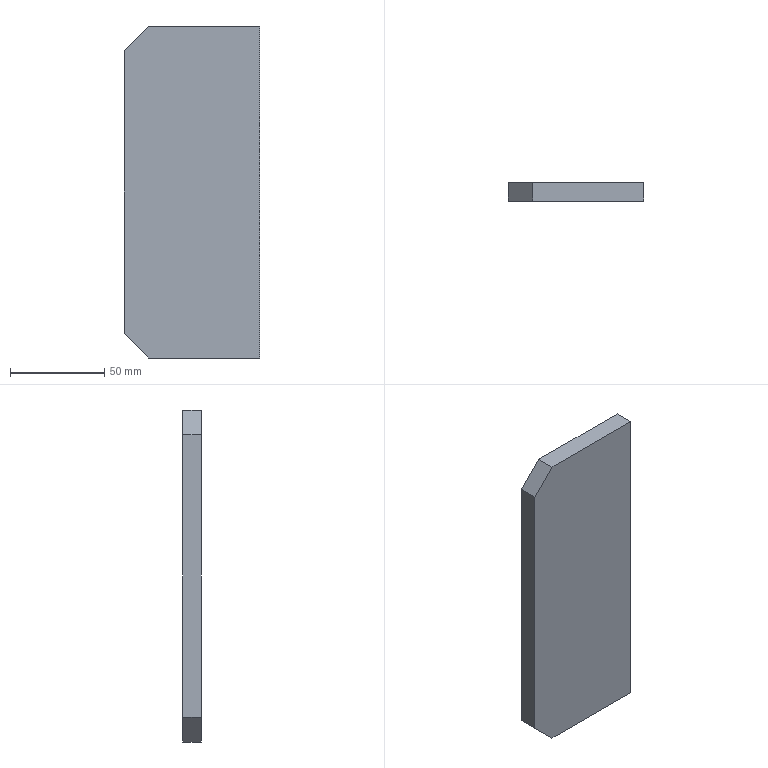Part | STEP file | 立柱填充筋Plate-194×150 | 1 solid | 8 faces | box 72 x 10 x 176 mm | volume 125030 mm3 | plane 8
STEP:
#1=CARTESIAN_POINT('',(0.,0.,0.));
#2=DIRECTION('',(0.,0.,1.));
#3=DIRECTION('',(1.,0.,0.));
#4=AXIS2_PLACEMENT_3D('',#1,#2,#3);
#5=CARTESIAN_POINT('',(72.,0.,88.));
#6=VERTEX_POINT('',#5);
#7=CARTESIAN_POINT('',(72.,0.,-88.));
#8=VERTEX_POINT('',#7);
#9=CARTESIAN_POINT('',(72.,0.,-88.));
#10=DIRECTION('',(0.,0.,-1.));
#11=VECTOR('',#10,1.);
#12=LINE('',#9,#11);
#13=CARTESIAN_POINT('',(72.,10.,-88.));
#14=DIRECTION('',(-1.,0.,0.));
#15=DIRECTION('',(0.,0.,1.));
#16=AXIS2_PLACEMENT_3D('',#13,#14,#15);
#17=PLANE('',#16);
#18=CARTESIAN_POINT('',(0.,-10.));
#19=DIRECTION('',(-1.,0.));
#20=VECTOR('',#19,1.);
#21=LINE('',#18,#20);
#22=(GEOMETRIC_REPRESENTATION_CONTEXT(2)PARAMETRIC_REPRESENTATION_CONTEXT()REPRESENTATION_CONTEXT('',''));
#23=DEFINITIONAL_REPRESENTATION('',(#21),#22);
#24=PCURVE('',#17,#23);
#25=CARTESIAN_POINT('',(0.,0.,0.));
#26=DIRECTION('',(0.,-1.,0.));
#27=DIRECTION('',(0.,0.,-1.));
#28=AXIS2_PLACEMENT_3D('',#25,#26,#27);
#29=PLANE('',#28);
#30=CARTESIAN_POINT('',(88.,72.));
#31=DIRECTION('',(1.,0.));
#32=VECTOR('',#31,1.);
#33=LINE('',#30,#32);
#34=(GEOMETRIC_REPRESENTATION_CONTEXT(2)PARAMETRIC_REPRESENTATION_CONTEXT()REPRESENTATION_CONTEXT('',''));
#35=DEFINITIONAL_REPRESENTATION('',(#33),#34);
#36=PCURVE('',#29,#35);
#37=SURFACE_CURVE('',#12,(#24,#36),.PCURVE_S1.);
#38=EDGE_CURVE('',#6,#8,#37,.T.);
#39=ORIENTED_EDGE('',*,*,#38,.T.);
#40=CARTESIAN_POINT('',(72.,10.,-88.));
#41=VERTEX_POINT('',#40);
#42=CARTESIAN_POINT('',(72.,10.,-88.));
#43=DIRECTION('',(0.,-1.,0.));
#44=VECTOR('',#43,1.);
#45=LINE('',#42,#44);
#46=CARTESIAN_POINT('',(0.,0.));
#47=DIRECTION('',(0.,-1.));
#48=VECTOR('',#47,1.);
#49=LINE('',#46,#48);
#50=(GEOMETRIC_REPRESENTATION_CONTEXT(2)PARAMETRIC_REPRESENTATION_CONTEXT()REPRESENTATION_CONTEXT('',''));
#51=DEFINITIONAL_REPRESENTATION('',(#49),#50);
#52=PCURVE('',#17,#51);
#53=CARTESIAN_POINT('',(0.,10.,-88.));
#54=DIRECTION('',(0.,0.,1.));
#55=DIRECTION('',(1.,0.,0.));
#56=AXIS2_PLACEMENT_3D('',#53,#54,#55);
#57=PLANE('',#56);
#58=CARTESIAN_POINT('',(72.,0.));
#59=DIRECTION('',(0.,-1.));
#60=VECTOR('',#59,1.);
#61=LINE('',#58,#60);
#62=(GEOMETRIC_REPRESENTATION_CONTEXT(2)PARAMETRIC_REPRESENTATION_CONTEXT()REPRESENTATION_CONTEXT('',''));
#63=DEFINITIONAL_REPRESENTATION('',(#61),#62);
#64=PCURVE('',#57,#63);
#65=SURFACE_CURVE('',#45,(#52,#64),.PCURVE_S1.);
#66=EDGE_CURVE('',#41,#8,#65,.T.);
#67=ORIENTED_EDGE('',*,*,#66,.F.);
#68=CARTESIAN_POINT('',(72.,10.,88.));
#69=VERTEX_POINT('',#68);
#70=CARTESIAN_POINT('',(72.,10.,-88.));
#71=DIRECTION('',(0.,0.,-1.));
#72=VECTOR('',#71,1.);
#73=LINE('',#70,#72);
#74=CARTESIAN_POINT('',(0.,0.));
#75=DIRECTION('',(-1.,0.));
#76=VECTOR('',#75,1.);
#77=LINE('',#74,#76);
#78=(GEOMETRIC_REPRESENTATION_CONTEXT(2)PARAMETRIC_REPRESENTATION_CONTEXT()REPRESENTATION_CONTEXT('',''));
#79=DEFINITIONAL_REPRESENTATION('',(#77),#78);
#80=PCURVE('',#17,#79);
#81=CARTESIAN_POINT('',(0.,10.,0.));
#82=DIRECTION('',(0.,-1.,0.));
#83=DIRECTION('',(0.,0.,-1.));
#84=AXIS2_PLACEMENT_3D('',#81,#82,#83);
#85=PLANE('',#84);
#86=CARTESIAN_POINT('',(88.,72.));
#87=DIRECTION('',(1.,0.));
#88=VECTOR('',#87,1.);
#89=LINE('',#86,#88);
#90=(GEOMETRIC_REPRESENTATION_CONTEXT(2)PARAMETRIC_REPRESENTATION_CONTEXT()REPRESENTATION_CONTEXT('',''));
#91=DEFINITIONAL_REPRESENTATION('',(#89),#90);
#92=PCURVE('',#85,#91);
#93=SURFACE_CURVE('',#73,(#80,#92),.PCURVE_S1.);
#94=EDGE_CURVE('',#69,#41,#93,.T.);
#95=ORIENTED_EDGE('',*,*,#94,.F.);
#96=CARTESIAN_POINT('',(72.,10.,88.));
#97=DIRECTION('',(0.,-1.,0.));
#98=VECTOR('',#97,1.);
#99=LINE('',#96,#98);
#100=CARTESIAN_POINT('',(176.,0.));
#101=DIRECTION('',(0.,-1.));
#102=VECTOR('',#101,1.);
#103=LINE('',#100,#102);
#104=(GEOMETRIC_REPRESENTATION_CONTEXT(2)PARAMETRIC_REPRESENTATION_CONTEXT()REPRESENTATION_CONTEXT('',''));
#105=DEFINITIONAL_REPRESENTATION('',(#103),#104);
#106=PCURVE('',#17,#105);
#107=CARTESIAN_POINT('',(72.,10.,88.));
#108=DIRECTION('',(0.,0.,-1.));
#109=DIRECTION('',(-1.,0.,0.));
#110=AXIS2_PLACEMENT_3D('',#107,#108,#109);
#111=PLANE('',#110);
#112=CARTESIAN_POINT('',(0.,0.));
#113=DIRECTION('',(0.,-1.));
#114=VECTOR('',#113,1.);
#115=LINE('',#112,#114);
#116=(GEOMETRIC_REPRESENTATION_CONTEXT(2)PARAMETRIC_REPRESENTATION_CONTEXT()REPRESENTATION_CONTEXT('',''));
#117=DEFINITIONAL_REPRESENTATION('',(#115),#116);
#118=PCURVE('',#111,#117);
#119=SURFACE_CURVE('',#99,(#106,#118),.PCURVE_S1.);
#120=EDGE_CURVE('',#69,#6,#119,.T.);
#121=ORIENTED_EDGE('',*,*,#120,.T.);
#122=EDGE_LOOP('',(#39,#67,#95,#121));
#123=FACE_BOUND('',#122,.T.);
#124=ADVANCED_FACE('',(#123),#17,.F.);
#125=CARTESIAN_POINT('',(13.,0.,-88.));
#126=VERTEX_POINT('',#125);
#127=CARTESIAN_POINT('',(0.,0.,-88.));
#128=DIRECTION('',(-1.,0.,0.));
#129=VECTOR('',#128,1.);
#130=LINE('',#127,#129);
#131=CARTESIAN_POINT('',(0.,-10.));
#132=DIRECTION('',(-1.,0.));
#133=VECTOR('',#132,1.);
#134=LINE('',#131,#133);
#135=(GEOMETRIC_REPRESENTATION_CONTEXT(2)PARAMETRIC_REPRESENTATION_CONTEXT()REPRESENTATION_CONTEXT('',''));
#136=DEFINITIONAL_REPRESENTATION('',(#134),#135);
#137=PCURVE('',#57,#136);
#138=CARTESIAN_POINT('',(88.,0.));
#139=DIRECTION('',(0.,-1.));
#140=VECTOR('',#139,1.);
#141=LINE('',#138,#140);
#142=(GEOMETRIC_REPRESENTATION_CONTEXT(2)PARAMETRIC_REPRESENTATION_CONTEXT()REPRESENTATION_CONTEXT('',''));
#143=DEFINITIONAL_REPRESENTATION('',(#141),#142);
#144=PCURVE('',#29,#143);
#145=SURFACE_CURVE('',#130,(#137,#144),.PCURVE_S1.);
#146=EDGE_CURVE('',#8,#126,#145,.T.);
#147=ORIENTED_EDGE('',*,*,#146,.T.);
#148=CARTESIAN_POINT('',(13.,10.,-88.));
#149=VERTEX_POINT('',#148);
#150=CARTESIAN_POINT('',(13.,10.,-88.));
#151=DIRECTION('',(0.,1.,0.));
#152=VECTOR('',#151,1.);
#153=LINE('',#150,#152);
#154=CARTESIAN_POINT('',(13.,0.));
#155=DIRECTION('',(0.,1.));
#156=VECTOR('',#155,1.);
#157=LINE('',#154,#156);
#158=(GEOMETRIC_REPRESENTATION_CONTEXT(2)PARAMETRIC_REPRESENTATION_CONTEXT()REPRESENTATION_CONTEXT('',''));
#159=DEFINITIONAL_REPRESENTATION('',(#157),#158);
#160=PCURVE('',#57,#159);
#161=CARTESIAN_POINT('',(0.,10.,-75.));
#162=DIRECTION('',(0.7071,0.,0.7071));
#163=DIRECTION('',(0.,-1.,0.));
#164=AXIS2_PLACEMENT_3D('',#161,#162,#163);
#165=PLANE('',#164);
#166=CARTESIAN_POINT('',(0.,18.385));
#167=DIRECTION('',(-1.,0.));
#168=VECTOR('',#167,1.);
#169=LINE('',#166,#168);
#170=(GEOMETRIC_REPRESENTATION_CONTEXT(2)PARAMETRIC_REPRESENTATION_CONTEXT()REPRESENTATION_CONTEXT('',''));
#171=DEFINITIONAL_REPRESENTATION('',(#169),#170);
#172=PCURVE('',#165,#171);
#173=SURFACE_CURVE('',#153,(#160,#172),.PCURVE_S1.);
#174=EDGE_CURVE('',#126,#149,#173,.T.);
#175=ORIENTED_EDGE('',*,*,#174,.T.);
#176=CARTESIAN_POINT('',(0.,10.,-88.));
#177=DIRECTION('',(-1.,0.,0.));
#178=VECTOR('',#177,1.);
#179=LINE('',#176,#178);
#180=CARTESIAN_POINT('',(0.,0.));
#181=DIRECTION('',(-1.,0.));
#182=VECTOR('',#181,1.);
#183=LINE('',#180,#182);
#184=(GEOMETRIC_REPRESENTATION_CONTEXT(2)PARAMETRIC_REPRESENTATION_CONTEXT()REPRESENTATION_CONTEXT('',''));
#185=DEFINITIONAL_REPRESENTATION('',(#183),#184);
#186=PCURVE('',#57,#185);
#187=CARTESIAN_POINT('',(88.,0.));
#188=DIRECTION('',(0.,-1.));
#189=VECTOR('',#188,1.);
#190=LINE('',#187,#189);
#191=(GEOMETRIC_REPRESENTATION_CONTEXT(2)PARAMETRIC_REPRESENTATION_CONTEXT()REPRESENTATION_CONTEXT('',''));
#192=DEFINITIONAL_REPRESENTATION('',(#190),#191);
#193=PCURVE('',#85,#192);
#194=SURFACE_CURVE('',#179,(#186,#193),.PCURVE_S1.);
#195=EDGE_CURVE('',#41,#149,#194,.T.);
#196=ORIENTED_EDGE('',*,*,#195,.F.);
#197=ORIENTED_EDGE('',*,*,#66,.T.);
#198=EDGE_LOOP('',(#147,#175,#196,#197));
#199=FACE_BOUND('',#198,.T.);
#200=ADVANCED_FACE('',(#199),#57,.F.);
#201=CARTESIAN_POINT('',(0.,0.,-75.));
#202=VERTEX_POINT('',#201);
#203=CARTESIAN_POINT('',(0.,0.,75.));
#204=VERTEX_POINT('',#203);
#205=CARTESIAN_POINT('',(0.,0.,88.));
#206=DIRECTION('',(0.,0.,1.));
#207=VECTOR('',#206,1.);
#208=LINE('',#205,#207);
#209=CARTESIAN_POINT('',(0.,10.,88.));
#210=DIRECTION('',(1.,0.,0.));
#211=DIRECTION('',(0.,0.,-1.));
#212=AXIS2_PLACEMENT_3D('',#209,#210,#211);
#213=PLANE('',#212);
#214=CARTESIAN_POINT('',(0.,-10.));
#215=DIRECTION('',(-1.,0.));
#216=VECTOR('',#215,1.);
#217=LINE('',#214,#216);
#218=(GEOMETRIC_REPRESENTATION_CONTEXT(2)PARAMETRIC_REPRESENTATION_CONTEXT()REPRESENTATION_CONTEXT('',''));
#219=DEFINITIONAL_REPRESENTATION('',(#217),#218);
#220=PCURVE('',#213,#219);
#221=CARTESIAN_POINT('',(-88.,0.));
#222=DIRECTION('',(-1.,0.));
#223=VECTOR('',#222,1.);
#224=LINE('',#221,#223);
#225=(GEOMETRIC_REPRESENTATION_CONTEXT(2)PARAMETRIC_REPRESENTATION_CONTEXT()REPRESENTATION_CONTEXT('',''));
#226=DEFINITIONAL_REPRESENTATION('',(#224),#225);
#227=PCURVE('',#29,#226);
#228=SURFACE_CURVE('',#208,(#220,#227),.PCURVE_S1.);
#229=EDGE_CURVE('',#202,#204,#228,.T.);
#230=ORIENTED_EDGE('',*,*,#229,.T.);
#231=CARTESIAN_POINT('',(0.,10.,75.));
#232=VERTEX_POINT('',#231);
#233=CARTESIAN_POINT('',(0.,10.,75.));
#234=DIRECTION('',(0.,1.,0.));
#235=VECTOR('',#234,1.);
#236=LINE('',#233,#235);
#237=CARTESIAN_POINT('',(13.,0.));
#238=DIRECTION('',(0.,1.));
#239=VECTOR('',#238,1.);
#240=LINE('',#237,#239);
#241=(GEOMETRIC_REPRESENTATION_CONTEXT(2)PARAMETRIC_REPRESENTATION_CONTEXT()REPRESENTATION_CONTEXT('',''));
#242=DEFINITIONAL_REPRESENTATION('',(#240),#241);
#243=PCURVE('',#213,#242);
#244=CARTESIAN_POINT('',(13.,10.,88.));
#245=DIRECTION('',(0.7071,0.,-0.7071));
#246=DIRECTION('',(0.,-1.,0.));
#247=AXIS2_PLACEMENT_3D('',#244,#245,#246);
#248=PLANE('',#247);
#249=CARTESIAN_POINT('',(0.,18.385));
#250=DIRECTION('',(-1.,0.));
#251=VECTOR('',#250,1.);
#252=LINE('',#249,#251);
#253=(GEOMETRIC_REPRESENTATION_CONTEXT(2)PARAMETRIC_REPRESENTATION_CONTEXT()REPRESENTATION_CONTEXT('',''));
#254=DEFINITIONAL_REPRESENTATION('',(#252),#253);
#255=PCURVE('',#248,#254);
#256=SURFACE_CURVE('',#236,(#243,#255),.PCURVE_S1.);
#257=EDGE_CURVE('',#204,#232,#256,.T.);
#258=ORIENTED_EDGE('',*,*,#257,.T.);
#259=CARTESIAN_POINT('',(0.,10.,-75.));
#260=VERTEX_POINT('',#259);
#261=CARTESIAN_POINT('',(0.,10.,88.));
#262=DIRECTION('',(0.,0.,1.));
#263=VECTOR('',#262,1.);
#264=LINE('',#261,#263);
#265=CARTESIAN_POINT('',(0.,0.));
#266=DIRECTION('',(-1.,0.));
#267=VECTOR('',#266,1.);
#268=LINE('',#265,#267);
#269=(GEOMETRIC_REPRESENTATION_CONTEXT(2)PARAMETRIC_REPRESENTATION_CONTEXT()REPRESENTATION_CONTEXT('',''));
#270=DEFINITIONAL_REPRESENTATION('',(#268),#269);
#271=PCURVE('',#213,#270);
#272=CARTESIAN_POINT('',(-88.,0.));
#273=DIRECTION('',(-1.,0.));
#274=VECTOR('',#273,1.);
#275=LINE('',#272,#274);
#276=(GEOMETRIC_REPRESENTATION_CONTEXT(2)PARAMETRIC_REPRESENTATION_CONTEXT()REPRESENTATION_CONTEXT('',''));
#277=DEFINITIONAL_REPRESENTATION('',(#275),#276);
#278=PCURVE('',#85,#277);
#279=SURFACE_CURVE('',#264,(#271,#278),.PCURVE_S1.);
#280=EDGE_CURVE('',#260,#232,#279,.T.);
#281=ORIENTED_EDGE('',*,*,#280,.F.);
#282=CARTESIAN_POINT('',(0.,10.,-75.));
#283=DIRECTION('',(0.,-1.,0.));
#284=VECTOR('',#283,1.);
#285=LINE('',#282,#284);
#286=CARTESIAN_POINT('',(163.,0.));
#287=DIRECTION('',(0.,-1.));
#288=VECTOR('',#287,1.);
#289=LINE('',#286,#288);
#290=(GEOMETRIC_REPRESENTATION_CONTEXT(2)PARAMETRIC_REPRESENTATION_CONTEXT()REPRESENTATION_CONTEXT('',''));
#291=DEFINITIONAL_REPRESENTATION('',(#289),#290);
#292=PCURVE('',#213,#291);
#293=CARTESIAN_POINT('',(0.,0.));
#294=DIRECTION('',(1.,0.));
#295=VECTOR('',#294,1.);
#296=LINE('',#293,#295);
#297=(GEOMETRIC_REPRESENTATION_CONTEXT(2)PARAMETRIC_REPRESENTATION_CONTEXT()REPRESENTATION_CONTEXT('',''));
#298=DEFINITIONAL_REPRESENTATION('',(#296),#297);
#299=PCURVE('',#165,#298);
#300=SURFACE_CURVE('',#285,(#292,#299),.PCURVE_S1.);
#301=EDGE_CURVE('',#260,#202,#300,.T.);
#302=ORIENTED_EDGE('',*,*,#301,.T.);
#303=EDGE_LOOP('',(#230,#258,#281,#302));
#304=FACE_BOUND('',#303,.T.);
#305=ADVANCED_FACE('',(#304),#213,.F.);
#306=CARTESIAN_POINT('',(13.,10.,88.));
#307=VERTEX_POINT('',#306);
#308=CARTESIAN_POINT('',(72.,10.,88.));
#309=DIRECTION('',(1.,0.,0.));
#310=VECTOR('',#309,1.);
#311=LINE('',#308,#310);
#312=CARTESIAN_POINT('',(0.,0.));
#313=DIRECTION('',(-1.,0.));
#314=VECTOR('',#313,1.);
#315=LINE('',#312,#314);
#316=(GEOMETRIC_REPRESENTATION_CONTEXT(2)PARAMETRIC_REPRESENTATION_CONTEXT()REPRESENTATION_CONTEXT('',''));
#317=DEFINITIONAL_REPRESENTATION('',(#315),#316);
#318=PCURVE('',#111,#317);
#319=CARTESIAN_POINT('',(-88.,72.));
#320=DIRECTION('',(0.,1.));
#321=VECTOR('',#320,1.);
#322=LINE('',#319,#321);
#323=(GEOMETRIC_REPRESENTATION_CONTEXT(2)PARAMETRIC_REPRESENTATION_CONTEXT()REPRESENTATION_CONTEXT('',''));
#324=DEFINITIONAL_REPRESENTATION('',(#322),#323);
#325=PCURVE('',#85,#324);
#326=SURFACE_CURVE('',#311,(#318,#325),.PCURVE_S1.);
#327=EDGE_CURVE('',#307,#69,#326,.T.);
#328=ORIENTED_EDGE('',*,*,#327,.F.);
#329=CARTESIAN_POINT('',(13.,0.,88.));
#330=VERTEX_POINT('',#329);
#331=CARTESIAN_POINT('',(13.,10.,88.));
#332=DIRECTION('',(0.,-1.,0.));
#333=VECTOR('',#332,1.);
#334=LINE('',#331,#333);
#335=CARTESIAN_POINT('',(59.,0.));
#336=DIRECTION('',(0.,-1.));
#337=VECTOR('',#336,1.);
#338=LINE('',#335,#337);
#339=(GEOMETRIC_REPRESENTATION_CONTEXT(2)PARAMETRIC_REPRESENTATION_CONTEXT()REPRESENTATION_CONTEXT('',''));
#340=DEFINITIONAL_REPRESENTATION('',(#338),#339);
#341=PCURVE('',#111,#340);
#342=CARTESIAN_POINT('',(0.,0.));
#343=DIRECTION('',(1.,0.));
#344=VECTOR('',#343,1.);
#345=LINE('',#342,#344);
#346=(GEOMETRIC_REPRESENTATION_CONTEXT(2)PARAMETRIC_REPRESENTATION_CONTEXT()REPRESENTATION_CONTEXT('',''));
#347=DEFINITIONAL_REPRESENTATION('',(#345),#346);
#348=PCURVE('',#248,#347);
#349=SURFACE_CURVE('',#334,(#341,#348),.PCURVE_S1.);
#350=EDGE_CURVE('',#307,#330,#349,.T.);
#351=ORIENTED_EDGE('',*,*,#350,.T.);
#352=CARTESIAN_POINT('',(72.,0.,88.));
#353=DIRECTION('',(1.,0.,0.));
#354=VECTOR('',#353,1.);
#355=LINE('',#352,#354);
#356=CARTESIAN_POINT('',(0.,-10.));
#357=DIRECTION('',(-1.,0.));
#358=VECTOR('',#357,1.);
#359=LINE('',#356,#358);
#360=(GEOMETRIC_REPRESENTATION_CONTEXT(2)PARAMETRIC_REPRESENTATION_CONTEXT()REPRESENTATION_CONTEXT('',''));
#361=DEFINITIONAL_REPRESENTATION('',(#359),#360);
#362=PCURVE('',#111,#361);
#363=CARTESIAN_POINT('',(-88.,72.));
#364=DIRECTION('',(0.,1.));
#365=VECTOR('',#364,1.);
#366=LINE('',#363,#365);
#367=(GEOMETRIC_REPRESENTATION_CONTEXT(2)PARAMETRIC_REPRESENTATION_CONTEXT()REPRESENTATION_CONTEXT('',''));
#368=DEFINITIONAL_REPRESENTATION('',(#366),#367);
#369=PCURVE('',#29,#368);
#370=SURFACE_CURVE('',#355,(#362,#369),.PCURVE_S1.);
#371=EDGE_CURVE('',#330,#6,#370,.T.);
#372=ORIENTED_EDGE('',*,*,#371,.T.);
#373=ORIENTED_EDGE('',*,*,#120,.F.);
#374=EDGE_LOOP('',(#328,#351,#372,#373));
#375=FACE_BOUND('',#374,.T.);
#376=ADVANCED_FACE('',(#375),#111,.F.);
#377=ORIENTED_EDGE('',*,*,#280,.T.);
#378=CARTESIAN_POINT('',(13.,10.,88.));
#379=DIRECTION('',(0.7071,0.,0.7071));
#380=VECTOR('',#379,1.);
#381=LINE('',#378,#380);
#382=CARTESIAN_POINT('',(-88.,13.));
#383=DIRECTION('',(-0.7071,0.7071));
#384=VECTOR('',#383,1.);
#385=LINE('',#382,#384);
#386=(GEOMETRIC_REPRESENTATION_CONTEXT(2)PARAMETRIC_REPRESENTATION_CONTEXT()REPRESENTATION_CONTEXT('',''));
#387=DEFINITIONAL_REPRESENTATION('',(#385),#386);
#388=PCURVE('',#85,#387);
#389=CARTESIAN_POINT('',(0.,0.));
#390=DIRECTION('',(0.,-1.));
#391=VECTOR('',#390,1.);
#392=LINE('',#389,#391);
#393=(GEOMETRIC_REPRESENTATION_CONTEXT(2)PARAMETRIC_REPRESENTATION_CONTEXT()REPRESENTATION_CONTEXT('',''));
#394=DEFINITIONAL_REPRESENTATION('',(#392),#393);
#395=PCURVE('',#248,#394);
#396=SURFACE_CURVE('',#381,(#388,#395),.PCURVE_S1.);
#397=EDGE_CURVE('',#232,#307,#396,.T.);
#398=ORIENTED_EDGE('',*,*,#397,.T.);
#399=ORIENTED_EDGE('',*,*,#327,.T.);
#400=ORIENTED_EDGE('',*,*,#94,.T.);
#401=ORIENTED_EDGE('',*,*,#195,.T.);
#402=CARTESIAN_POINT('',(0.,10.,-75.));
#403=DIRECTION('',(-0.7071,0.,0.7071));
#404=VECTOR('',#403,1.);
#405=LINE('',#402,#404);
#406=CARTESIAN_POINT('',(75.,0.));
#407=DIRECTION('',(-0.7071,-0.7071));
#408=VECTOR('',#407,1.);
#409=LINE('',#406,#408);
#410=(GEOMETRIC_REPRESENTATION_CONTEXT(2)PARAMETRIC_REPRESENTATION_CONTEXT()REPRESENTATION_CONTEXT('',''));
#411=DEFINITIONAL_REPRESENTATION('',(#409),#410);
#412=PCURVE('',#85,#411);
#413=CARTESIAN_POINT('',(0.,0.));
#414=DIRECTION('',(0.,-1.));
#415=VECTOR('',#414,1.);
#416=LINE('',#413,#415);
#417=(GEOMETRIC_REPRESENTATION_CONTEXT(2)PARAMETRIC_REPRESENTATION_CONTEXT()REPRESENTATION_CONTEXT('',''));
#418=DEFINITIONAL_REPRESENTATION('',(#416),#417);
#419=PCURVE('',#165,#418);
#420=SURFACE_CURVE('',#405,(#412,#419),.PCURVE_S1.);
#421=EDGE_CURVE('',#149,#260,#420,.T.);
#422=ORIENTED_EDGE('',*,*,#421,.T.);
#423=EDGE_LOOP('',(#377,#398,#399,#400,#401,#422));
#424=FACE_BOUND('',#423,.T.);
#425=ADVANCED_FACE('',(#424),#85,.F.);
#426=ORIENTED_EDGE('',*,*,#371,.F.);
#427=CARTESIAN_POINT('',(-37.5,0.,37.5));
#428=DIRECTION('',(-0.7071,0.,-0.7071));
#429=VECTOR('',#428,1.);
#430=LINE('',#427,#429);
#431=CARTESIAN_POINT('',(-37.5,-37.5));
#432=DIRECTION('',(0.7071,-0.7071));
#433=VECTOR('',#432,1.);
#434=LINE('',#431,#433);
#435=(GEOMETRIC_REPRESENTATION_CONTEXT(2)PARAMETRIC_REPRESENTATION_CONTEXT()REPRESENTATION_CONTEXT('',''));
#436=DEFINITIONAL_REPRESENTATION('',(#434),#435);
#437=PCURVE('',#29,#436);
#438=CARTESIAN_POINT('',(10.,71.418));
#439=DIRECTION('',(0.,1.));
#440=VECTOR('',#439,1.);
#441=LINE('',#438,#440);
#442=(GEOMETRIC_REPRESENTATION_CONTEXT(2)PARAMETRIC_REPRESENTATION_CONTEXT()REPRESENTATION_CONTEXT('',''));
#443=DEFINITIONAL_REPRESENTATION('',(#441),#442);
#444=PCURVE('',#248,#443);
#445=SURFACE_CURVE('',#430,(#437,#444),.PCURVE_S1.);
#446=EDGE_CURVE('',#330,#204,#445,.T.);
#447=ORIENTED_EDGE('',*,*,#446,.T.);
#448=ORIENTED_EDGE('',*,*,#229,.F.);
#449=CARTESIAN_POINT('',(-37.5,0.,-37.5));
#450=DIRECTION('',(0.7071,0.,-0.7071));
#451=VECTOR('',#450,1.);
#452=LINE('',#449,#451);
#453=CARTESIAN_POINT('',(37.5,-37.5));
#454=DIRECTION('',(0.7071,0.7071));
#455=VECTOR('',#454,1.);
#456=LINE('',#453,#455);
#457=(GEOMETRIC_REPRESENTATION_CONTEXT(2)PARAMETRIC_REPRESENTATION_CONTEXT()REPRESENTATION_CONTEXT('',''));
#458=DEFINITIONAL_REPRESENTATION('',(#456),#457);
#459=PCURVE('',#29,#458);
#460=CARTESIAN_POINT('',(10.,-53.033));
#461=DIRECTION('',(0.,1.));
#462=VECTOR('',#461,1.);
#463=LINE('',#460,#462);
#464=(GEOMETRIC_REPRESENTATION_CONTEXT(2)PARAMETRIC_REPRESENTATION_CONTEXT()REPRESENTATION_CONTEXT('',''));
#465=DEFINITIONAL_REPRESENTATION('',(#463),#464);
#466=PCURVE('',#165,#465);
#467=SURFACE_CURVE('',#452,(#459,#466),.PCURVE_S1.);
#468=EDGE_CURVE('',#202,#126,#467,.T.);
#469=ORIENTED_EDGE('',*,*,#468,.T.);
#470=ORIENTED_EDGE('',*,*,#146,.F.);
#471=ORIENTED_EDGE('',*,*,#38,.F.);
#472=EDGE_LOOP('',(#426,#447,#448,#469,#470,#471));
#473=FACE_BOUND('',#472,.T.);
#474=ADVANCED_FACE('',(#473),#29,.T.);
#475=ORIENTED_EDGE('',*,*,#397,.F.);
#476=ORIENTED_EDGE('',*,*,#257,.F.);
#477=ORIENTED_EDGE('',*,*,#446,.F.);
#478=ORIENTED_EDGE('',*,*,#350,.F.);
#479=EDGE_LOOP('',(#475,#476,#477,#478));
#480=FACE_BOUND('',#479,.T.);
#481=ADVANCED_FACE('',(#480),#248,.F.);
#482=ORIENTED_EDGE('',*,*,#421,.F.);
#483=ORIENTED_EDGE('',*,*,#174,.F.);
#484=ORIENTED_EDGE('',*,*,#468,.F.);
#485=ORIENTED_EDGE('',*,*,#301,.F.);
#486=EDGE_LOOP('',(#482,#483,#484,#485));
#487=FACE_BOUND('',#486,.T.);
#488=ADVANCED_FACE('',(#487),#165,.F.);
#489=CLOSED_SHELL('',(#124,#200,#305,#376,#425,#474,#481,#488));
#490=MANIFOLD_SOLID_BREP('',#489);
#491=(LENGTH_UNIT()NAMED_UNIT(*)SI_UNIT(.MILLI.,.METRE.));
#492=UNCERTAINTY_MEASURE_WITH_UNIT(LENGTH_MEASURE(0.0000001),#491,'','');
#493=(NAMED_UNIT(*)PLANE_ANGLE_UNIT()SI_UNIT($,.RADIAN.));
#494=(NAMED_UNIT(*)SI_UNIT($,.STERADIAN.)SOLID_ANGLE_UNIT());
#495=(GEOMETRIC_REPRESENTATION_CONTEXT(3)GLOBAL_UNCERTAINTY_ASSIGNED_CONTEXT((#492))GLOBAL_UNIT_ASSIGNED_CONTEXT((#491,#493,#494))REPRESENTATION_CONTEXT('',''));
#496=ADVANCED_BREP_SHAPE_REPRESENTATION('',(#4,#490),#495);